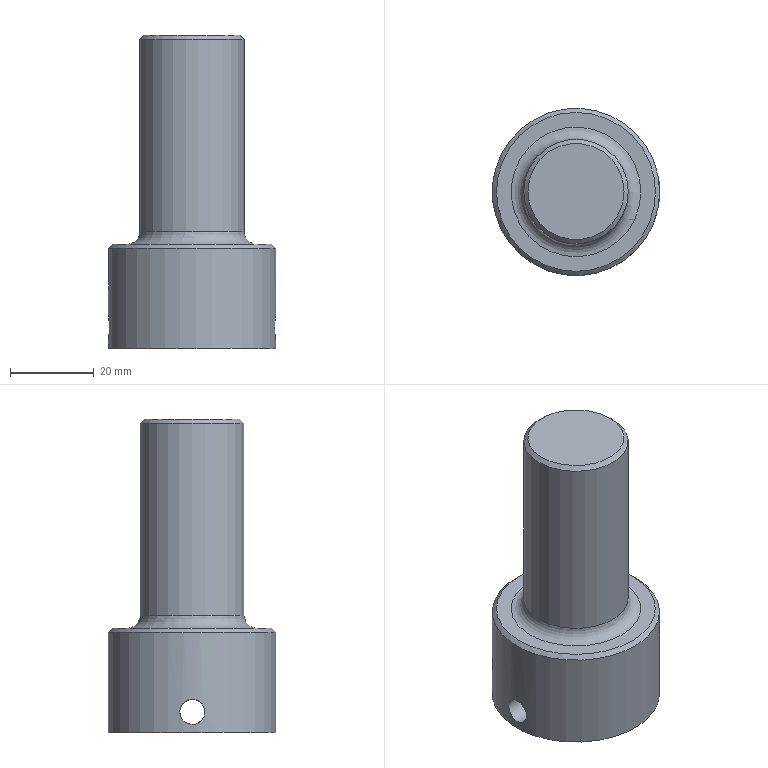Part | NX | features DATUM_CSYS 5, EXTRUDE 4, SKETCH 4, CHAMFER 2, BLEND 1 | 1 solid | 15 faces | box 40 x 40 x 75 mm | volume 54175 mm3 | plane 8 | cylinder 4 | cone 2 | torus 1 | commonest cylinder face diameters 6 x2 25 x1 40 x1
STEP:
#1=CARTESIAN_POINT('',(20.,0.,2.001));
#2=VERTEX_POINT('',#1);
#3=CARTESIAN_POINT('',(19.887,-2.373,2.578));
#4=CARTESIAN_POINT('',(20.056,0.01073,1.676));
#5=CARTESIAN_POINT('',(19.888,2.33,2.726));
#6=CARTESIAN_POINT('',(19.733,3.228,5.103));
#7=CARTESIAN_POINT('',(19.909,2.181,7.424));
#8=CARTESIAN_POINT('',(20.055,-0.2011,8.322));
#9=CARTESIAN_POINT('',(19.865,-2.516,7.277));
#10=CARTESIAN_POINT('',(19.701,-3.418,4.897));
#11=CARTESIAN_POINT('',(19.887,-2.373,2.578));
#12=CARTESIAN_POINT('',(20.056,0.01073,1.676));
#13=CARTESIAN_POINT('',(19.888,2.33,2.726));
#14=B_SPLINE_CURVE_WITH_KNOTS('',3,(#3,#4,#5,#6,#7,#8,#9,#10,#11,#12,#13),.UNSPECIFIED.,.T.,.F.,(1,1,1,1,1,1,1,1,1,1,1,1,1,1,1),(-0.007044,-0.004696,-0.002348,0.,0.002348,0.004696,0.007044,0.009392,0.01174,0.01409,0.01644,0.01878,0.02113,0.02348,0.02583),.UNSPECIFIED.);
#15=EDGE_CURVE('',#2,#2,#14,.T.);
#16=ORIENTED_EDGE('',*,*,#15,.F.);
#17=EDGE_LOOP('',(#16));
#18=FACE_BOUND('',#17,.T.);
#19=CARTESIAN_POINT('',(-20.,-0.0948,2.));
#20=VERTEX_POINT('',#19);
#21=CARTESIAN_POINT('',(-19.898,2.259,2.651));
#22=CARTESIAN_POINT('',(-20.056,-0.09565,1.675));
#23=CARTESIAN_POINT('',(-19.876,-2.445,2.65));
#24=CARTESIAN_POINT('',(-19.701,-3.419,4.996));
#25=CARTESIAN_POINT('',(-19.876,-2.447,7.35));
#26=CARTESIAN_POINT('',(-20.056,-0.09747,8.324));
#27=CARTESIAN_POINT('',(-19.899,2.253,7.354));
#28=CARTESIAN_POINT('',(-19.733,3.23,5.004));
#29=CARTESIAN_POINT('',(-19.898,2.259,2.651));
#30=CARTESIAN_POINT('',(-20.056,-0.09565,1.675));
#31=CARTESIAN_POINT('',(-19.876,-2.445,2.65));
#32=B_SPLINE_CURVE_WITH_KNOTS('',3,(#21,#22,#23,#24,#25,#26,#27,#28,#29,#30,#31),.UNSPECIFIED.,.T.,.F.,(1,1,1,1,1,1,1,1,1,1,1,1,1,1,1),(-0.007044,-0.004696,-0.002348,0.,0.002348,0.004696,0.007044,0.009391,0.01174,0.01409,0.01644,0.01878,0.02113,0.02348,0.02583),.UNSPECIFIED.);
#33=EDGE_CURVE('',#20,#20,#32,.T.);
#34=ORIENTED_EDGE('',*,*,#33,.F.);
#35=EDGE_LOOP('',(#34));
#36=FACE_BOUND('',#35,.T.);
#37=CARTESIAN_POINT('',(20.,0.,24.));
#38=VERTEX_POINT('',#37);
#39=CARTESIAN_POINT('',(0.,0.,24.));
#40=DIRECTION('',(0.,0.,1.));
#41=DIRECTION('',(1.,0.,0.));
#42=AXIS2_PLACEMENT_3D('',#39,#40,#41);
#43=CIRCLE('',#42,20.);
#44=EDGE_CURVE('',#38,#38,#43,.F.);
#45=ORIENTED_EDGE('',*,*,#44,.T.);
#46=EDGE_LOOP('',(#45));
#47=FACE_BOUND('',#46,.T.);
#48=CARTESIAN_POINT('',(20.,0.,0.));
#49=VERTEX_POINT('',#48);
#50=CARTESIAN_POINT('',(0.,0.,0.));
#51=DIRECTION('',(0.,0.,1.));
#52=DIRECTION('',(1.,0.,0.));
#53=AXIS2_PLACEMENT_3D('',#50,#51,#52);
#54=CIRCLE('',#53,20.);
#55=EDGE_CURVE('',#49,#49,#54,.T.);
#56=ORIENTED_EDGE('',*,*,#55,.T.);
#57=EDGE_LOOP('',(#56));
#58=FACE_BOUND('',#57,.T.);
#59=CARTESIAN_POINT('',(0.,0.,0.));
#60=DIRECTION('',(0.,0.,1.));
#61=DIRECTION('',(1.,0.,0.));
#62=AXIS2_PLACEMENT_3D('',#59,#60,#61);
#63=CYLINDRICAL_SURFACE('',#62,20.);
#64=ADVANCED_FACE('',(#18,#36,#47,#58),#63,.T.);
#65=CARTESIAN_POINT('',(5.,5.,0.));
#66=VERTEX_POINT('',#65);
#67=CARTESIAN_POINT('',(-5.,5.,0.));
#68=VERTEX_POINT('',#67);
#69=CARTESIAN_POINT('',(5.,5.,0.));
#70=DIRECTION('',(-1.,0.,0.));
#71=VECTOR('',#70,1000.);
#72=LINE('',#69,#71);
#73=EDGE_CURVE('',#66,#68,#72,.T.);
#74=ORIENTED_EDGE('',*,*,#73,.T.);
#75=CARTESIAN_POINT('',(-5.,-5.,0.));
#76=VERTEX_POINT('',#75);
#77=CARTESIAN_POINT('',(-5.,5.,0.));
#78=DIRECTION('',(0.,-1.,0.));
#79=VECTOR('',#78,1000.);
#80=LINE('',#77,#79);
#81=EDGE_CURVE('',#68,#76,#80,.T.);
#82=ORIENTED_EDGE('',*,*,#81,.T.);
#83=CARTESIAN_POINT('',(5.,-5.,0.));
#84=VERTEX_POINT('',#83);
#85=CARTESIAN_POINT('',(-5.,-5.,0.));
#86=DIRECTION('',(1.,0.,0.));
#87=VECTOR('',#86,1000.);
#88=LINE('',#85,#87);
#89=EDGE_CURVE('',#76,#84,#88,.T.);
#90=ORIENTED_EDGE('',*,*,#89,.T.);
#91=CARTESIAN_POINT('',(5.,-5.,0.));
#92=DIRECTION('',(0.,1.,0.));
#93=VECTOR('',#92,1000.);
#94=LINE('',#91,#93);
#95=EDGE_CURVE('',#84,#66,#94,.T.);
#96=ORIENTED_EDGE('',*,*,#95,.T.);
#97=EDGE_LOOP('',(#74,#82,#90,#96));
#98=FACE_BOUND('',#97,.T.);
#99=ORIENTED_EDGE('',*,*,#55,.F.);
#100=EDGE_LOOP('',(#99));
#101=FACE_BOUND('',#100,.T.);
#102=CARTESIAN_POINT('',(0.,0.,0.));
#103=DIRECTION('',(0.,0.,1.));
#104=DIRECTION('',(1.,0.,0.));
#105=AXIS2_PLACEMENT_3D('',#102,#103,#104);
#106=PLANE('',#105);
#107=ADVANCED_FACE('',(#98,#101),#106,.F.);
#108=CARTESIAN_POINT('',(15.5,0.,25.));
#109=VERTEX_POINT('',#108);
#110=CARTESIAN_POINT('',(0.,0.,25.));
#111=DIRECTION('',(0.,0.,1.));
#112=DIRECTION('',(1.,0.,0.));
#113=AXIS2_PLACEMENT_3D('',#110,#111,#112);
#114=CIRCLE('',#113,15.5);
#115=EDGE_CURVE('',#109,#109,#114,.F.);
#116=ORIENTED_EDGE('',*,*,#115,.T.);
#117=EDGE_LOOP('',(#116));
#118=FACE_BOUND('',#117,.T.);
#119=CARTESIAN_POINT('',(19.,0.,25.));
#120=VERTEX_POINT('',#119);
#121=CARTESIAN_POINT('',(0.,0.,25.));
#122=DIRECTION('',(0.,0.,1.));
#123=DIRECTION('',(1.,0.,0.));
#124=AXIS2_PLACEMENT_3D('',#121,#122,#123);
#125=CIRCLE('',#124,19.);
#126=EDGE_CURVE('',#120,#120,#125,.T.);
#127=ORIENTED_EDGE('',*,*,#126,.T.);
#128=EDGE_LOOP('',(#127));
#129=FACE_BOUND('',#128,.T.);
#130=CARTESIAN_POINT('',(0.,0.,25.));
#131=DIRECTION('',(0.,0.,1.));
#132=DIRECTION('',(1.,0.,0.));
#133=AXIS2_PLACEMENT_3D('',#130,#131,#132);
#134=PLANE('',#133);
#135=ADVANCED_FACE('',(#118,#129),#134,.T.);
#136=ORIENTED_EDGE('',*,*,#44,.F.);
#137=EDGE_LOOP('',(#136));
#138=FACE_BOUND('',#137,.T.);
#139=ORIENTED_EDGE('',*,*,#126,.F.);
#140=EDGE_LOOP('',(#139));
#141=FACE_BOUND('',#140,.T.);
#142=CARTESIAN_POINT('',(0.,0.,25.));
#143=DIRECTION('',(0.,0.,-1.));
#144=DIRECTION('',(-1.,0.,0.));
#145=AXIS2_PLACEMENT_3D('',#142,#143,#144);
#146=CONICAL_SURFACE('',#145,19.,0.7854);
#147=ADVANCED_FACE('',(#138,#141),#146,.T.);
#148=CARTESIAN_POINT('',(-5.,-3.095,5.));
#149=VERTEX_POINT('',#148);
#150=CARTESIAN_POINT('',(-5.,-0.0948,5.));
#151=DIRECTION('',(-1.,0.,0.));
#152=DIRECTION('',(0.,-1.,0.));
#153=AXIS2_PLACEMENT_3D('',#150,#151,#152);
#154=CIRCLE('',#153,3.);
#155=EDGE_CURVE('',#149,#149,#154,.T.);
#156=ORIENTED_EDGE('',*,*,#155,.T.);
#157=EDGE_LOOP('',(#156));
#158=FACE_BOUND('',#157,.T.);
#159=CARTESIAN_POINT('',(-5.,-5.,10.));
#160=VERTEX_POINT('',#159);
#161=CARTESIAN_POINT('',(-5.,5.,10.));
#162=VERTEX_POINT('',#161);
#163=CARTESIAN_POINT('',(-5.,5.,10.));
#164=DIRECTION('',(0.,-1.,0.));
#165=VECTOR('',#164,1000.);
#166=LINE('',#163,#165);
#167=EDGE_CURVE('',#160,#162,#166,.F.);
#168=ORIENTED_EDGE('',*,*,#167,.F.);
#169=CARTESIAN_POINT('',(-5.,-5.,0.));
#170=DIRECTION('',(0.,0.,1.));
#171=VECTOR('',#170,1000.);
#172=LINE('',#169,#171);
#173=EDGE_CURVE('',#160,#76,#172,.F.);
#174=ORIENTED_EDGE('',*,*,#173,.T.);
#175=ORIENTED_EDGE('',*,*,#81,.F.);
#176=CARTESIAN_POINT('',(-5.,5.,0.));
#177=DIRECTION('',(0.,0.,1.));
#178=VECTOR('',#177,1000.);
#179=LINE('',#176,#178);
#180=EDGE_CURVE('',#162,#68,#179,.F.);
#181=ORIENTED_EDGE('',*,*,#180,.F.);
#182=EDGE_LOOP('',(#168,#174,#175,#181));
#183=FACE_BOUND('',#182,.T.);
#184=CARTESIAN_POINT('',(-5.,5.,0.));
#185=DIRECTION('',(-1.,0.,0.));
#186=DIRECTION('',(0.,-1.,0.));
#187=AXIS2_PLACEMENT_3D('',#184,#185,#186);
#188=PLANE('',#187);
#189=ADVANCED_FACE('',(#158,#183),#188,.F.);
#190=CARTESIAN_POINT('',(5.,-5.,10.));
#191=VERTEX_POINT('',#190);
#192=CARTESIAN_POINT('',(-5.,-5.,10.));
#193=DIRECTION('',(1.,0.,0.));
#194=VECTOR('',#193,1000.);
#195=LINE('',#192,#194);
#196=EDGE_CURVE('',#191,#160,#195,.F.);
#197=ORIENTED_EDGE('',*,*,#196,.F.);
#198=CARTESIAN_POINT('',(5.,-5.,0.));
#199=DIRECTION('',(0.,0.,1.));
#200=VECTOR('',#199,1000.);
#201=LINE('',#198,#200);
#202=EDGE_CURVE('',#191,#84,#201,.F.);
#203=ORIENTED_EDGE('',*,*,#202,.T.);
#204=ORIENTED_EDGE('',*,*,#89,.F.);
#205=ORIENTED_EDGE('',*,*,#173,.F.);
#206=EDGE_LOOP('',(#197,#203,#204,#205));
#207=FACE_BOUND('',#206,.T.);
#208=CARTESIAN_POINT('',(-5.,-5.,0.));
#209=DIRECTION('',(0.,-1.,0.));
#210=DIRECTION('',(1.,0.,0.));
#211=AXIS2_PLACEMENT_3D('',#208,#209,#210);
#212=PLANE('',#211);
#213=ADVANCED_FACE('',(#207),#212,.F.);
#214=CARTESIAN_POINT('',(5.,2.905,5.));
#215=VERTEX_POINT('',#214);
#216=CARTESIAN_POINT('',(5.,-0.0948,5.));
#217=DIRECTION('',(1.,0.,0.));
#218=DIRECTION('',(0.,1.,0.));
#219=AXIS2_PLACEMENT_3D('',#216,#217,#218);
#220=CIRCLE('',#219,3.);
#221=EDGE_CURVE('',#215,#215,#220,.T.);
#222=ORIENTED_EDGE('',*,*,#221,.T.);
#223=EDGE_LOOP('',(#222));
#224=FACE_BOUND('',#223,.T.);
#225=CARTESIAN_POINT('',(5.,5.,10.));
#226=VERTEX_POINT('',#225);
#227=CARTESIAN_POINT('',(5.,-5.,10.));
#228=DIRECTION('',(0.,1.,0.));
#229=VECTOR('',#228,1000.);
#230=LINE('',#227,#229);
#231=EDGE_CURVE('',#226,#191,#230,.F.);
#232=ORIENTED_EDGE('',*,*,#231,.F.);
#233=CARTESIAN_POINT('',(5.,5.,0.));
#234=DIRECTION('',(0.,0.,1.));
#235=VECTOR('',#234,1000.);
#236=LINE('',#233,#235);
#237=EDGE_CURVE('',#226,#66,#236,.F.);
#238=ORIENTED_EDGE('',*,*,#237,.T.);
#239=ORIENTED_EDGE('',*,*,#95,.F.);
#240=ORIENTED_EDGE('',*,*,#202,.F.);
#241=EDGE_LOOP('',(#232,#238,#239,#240));
#242=FACE_BOUND('',#241,.T.);
#243=CARTESIAN_POINT('',(5.,-5.,0.));
#244=DIRECTION('',(1.,0.,0.));
#245=DIRECTION('',(0.,1.,0.));
#246=AXIS2_PLACEMENT_3D('',#243,#244,#245);
#247=PLANE('',#246);
#248=ADVANCED_FACE('',(#224,#242),#247,.F.);
#249=CARTESIAN_POINT('',(5.,5.,10.));
#250=DIRECTION('',(-1.,0.,0.));
#251=VECTOR('',#250,1000.);
#252=LINE('',#249,#251);
#253=EDGE_CURVE('',#162,#226,#252,.F.);
#254=ORIENTED_EDGE('',*,*,#253,.F.);
#255=ORIENTED_EDGE('',*,*,#180,.T.);
#256=ORIENTED_EDGE('',*,*,#73,.F.);
#257=ORIENTED_EDGE('',*,*,#237,.F.);
#258=EDGE_LOOP('',(#254,#255,#256,#257));
#259=FACE_BOUND('',#258,.T.);
#260=CARTESIAN_POINT('',(5.,5.,0.));
#261=DIRECTION('',(0.,1.,0.));
#262=DIRECTION('',(-1.,0.,0.));
#263=AXIS2_PLACEMENT_3D('',#260,#261,#262);
#264=PLANE('',#263);
#265=ADVANCED_FACE('',(#259),#264,.F.);
#266=ORIENTED_EDGE('',*,*,#167,.T.);
#267=ORIENTED_EDGE('',*,*,#253,.T.);
#268=ORIENTED_EDGE('',*,*,#231,.T.);
#269=ORIENTED_EDGE('',*,*,#196,.T.);
#270=EDGE_LOOP('',(#266,#267,#268,#269));
#271=FACE_BOUND('',#270,.T.);
#272=CARTESIAN_POINT('',(0.,0.,10.));
#273=DIRECTION('',(0.,0.,1.));
#274=DIRECTION('',(1.,0.,0.));
#275=AXIS2_PLACEMENT_3D('',#272,#273,#274);
#276=PLANE('',#275);
#277=ADVANCED_FACE('',(#271),#276,.F.);
#278=ORIENTED_EDGE('',*,*,#15,.T.);
#279=EDGE_LOOP('',(#278));
#280=FACE_BOUND('',#279,.T.);
#281=ORIENTED_EDGE('',*,*,#221,.F.);
#282=EDGE_LOOP('',(#281));
#283=FACE_BOUND('',#282,.T.);
#284=CARTESIAN_POINT('',(-24.5,-0.0948,5.));
#285=DIRECTION('',(1.,0.,0.));
#286=DIRECTION('',(0.,0.,-1.));
#287=AXIS2_PLACEMENT_3D('',#284,#285,#286);
#288=CYLINDRICAL_SURFACE('',#287,3.);
#289=ADVANCED_FACE('',(#280,#283),#288,.F.);
#290=ORIENTED_EDGE('',*,*,#33,.T.);
#291=EDGE_LOOP('',(#290));
#292=FACE_BOUND('',#291,.T.);
#293=ORIENTED_EDGE('',*,*,#155,.F.);
#294=EDGE_LOOP('',(#293));
#295=FACE_BOUND('',#294,.T.);
#296=CARTESIAN_POINT('',(-24.5,-0.0948,5.));
#297=DIRECTION('',(1.,0.,0.));
#298=DIRECTION('',(0.,0.,-1.));
#299=AXIS2_PLACEMENT_3D('',#296,#297,#298);
#300=CYLINDRICAL_SURFACE('',#299,3.);
#301=ADVANCED_FACE('',(#292,#295),#300,.F.);
#302=CARTESIAN_POINT('',(12.5,0.,74.));
#303=VERTEX_POINT('',#302);
#304=CARTESIAN_POINT('',(0.,0.,74.));
#305=DIRECTION('',(0.,0.,1.));
#306=DIRECTION('',(1.,0.,0.));
#307=AXIS2_PLACEMENT_3D('',#304,#305,#306);
#308=CIRCLE('',#307,12.5);
#309=EDGE_CURVE('',#303,#303,#308,.F.);
#310=ORIENTED_EDGE('',*,*,#309,.T.);
#311=EDGE_LOOP('',(#310));
#312=FACE_BOUND('',#311,.T.);
#313=CARTESIAN_POINT('',(12.5,0.,28.));
#314=VERTEX_POINT('',#313);
#315=CARTESIAN_POINT('',(0.,0.,28.));
#316=DIRECTION('',(0.,0.,1.));
#317=DIRECTION('',(1.,0.,0.));
#318=AXIS2_PLACEMENT_3D('',#315,#316,#317);
#319=CIRCLE('',#318,12.5);
#320=EDGE_CURVE('',#314,#314,#319,.T.);
#321=ORIENTED_EDGE('',*,*,#320,.T.);
#322=EDGE_LOOP('',(#321));
#323=FACE_BOUND('',#322,.T.);
#324=CARTESIAN_POINT('',(0.,0.,75.));
#325=DIRECTION('',(0.,0.,-1.));
#326=DIRECTION('',(-1.,0.,0.));
#327=AXIS2_PLACEMENT_3D('',#324,#325,#326);
#328=CYLINDRICAL_SURFACE('',#327,12.5);
#329=ADVANCED_FACE('',(#312,#323),#328,.T.);
#330=CARTESIAN_POINT('',(11.5,0.,75.));
#331=VERTEX_POINT('',#330);
#332=CARTESIAN_POINT('',(0.,0.,75.));
#333=DIRECTION('',(0.,0.,1.));
#334=DIRECTION('',(1.,0.,0.));
#335=AXIS2_PLACEMENT_3D('',#332,#333,#334);
#336=CIRCLE('',#335,11.5);
#337=EDGE_CURVE('',#331,#331,#336,.T.);
#338=ORIENTED_EDGE('',*,*,#337,.T.);
#339=EDGE_LOOP('',(#338));
#340=FACE_BOUND('',#339,.T.);
#341=CARTESIAN_POINT('',(0.,0.,75.));
#342=DIRECTION('',(0.,0.,1.));
#343=DIRECTION('',(1.,0.,0.));
#344=AXIS2_PLACEMENT_3D('',#341,#342,#343);
#345=PLANE('',#344);
#346=ADVANCED_FACE('',(#340),#345,.T.);
#347=ORIENTED_EDGE('',*,*,#115,.F.);
#348=EDGE_LOOP('',(#347));
#349=FACE_BOUND('',#348,.T.);
#350=ORIENTED_EDGE('',*,*,#320,.F.);
#351=EDGE_LOOP('',(#350));
#352=FACE_BOUND('',#351,.T.);
#353=CARTESIAN_POINT('',(0.,0.,28.));
#354=DIRECTION('',(0.,0.,1.));
#355=DIRECTION('',(1.,0.,0.));
#356=AXIS2_PLACEMENT_3D('',#353,#354,#355);
#357=TOROIDAL_SURFACE('',#356,15.5,3.);
#358=ADVANCED_FACE('',(#349,#352),#357,.F.);
#359=ORIENTED_EDGE('',*,*,#309,.F.);
#360=EDGE_LOOP('',(#359));
#361=FACE_BOUND('',#360,.T.);
#362=ORIENTED_EDGE('',*,*,#337,.F.);
#363=EDGE_LOOP('',(#362));
#364=FACE_BOUND('',#363,.T.);
#365=CARTESIAN_POINT('',(0.,0.,75.));
#366=DIRECTION('',(0.,0.,-1.));
#367=DIRECTION('',(-1.,0.,0.));
#368=AXIS2_PLACEMENT_3D('',#365,#366,#367);
#369=CONICAL_SURFACE('',#368,11.5,0.7854);
#370=ADVANCED_FACE('',(#361,#364),#369,.T.);
#371=CLOSED_SHELL('',(#64,#107,#135,#147,#189,#213,#248,#265,#277,#289,#301,#329,#346,#358,#370));
#372=MANIFOLD_SOLID_BREP('',#371);
#373=(LENGTH_UNIT()NAMED_UNIT(*)SI_UNIT(.MILLI.,.METRE.));
#374=UNCERTAINTY_MEASURE_WITH_UNIT(LENGTH_MEASURE(0.0508),#373,'','');
#375=(NAMED_UNIT(*)PLANE_ANGLE_UNIT()SI_UNIT($,.RADIAN.));
#376=(NAMED_UNIT(*)SI_UNIT($,.STERADIAN.)SOLID_ANGLE_UNIT());
#377=(GEOMETRIC_REPRESENTATION_CONTEXT(3)GLOBAL_UNCERTAINTY_ASSIGNED_CONTEXT((#374))GLOBAL_UNIT_ASSIGNED_CONTEXT((#373,#375,#376))REPRESENTATION_CONTEXT('',''));
#378=ADVANCED_BREP_SHAPE_REPRESENTATION('',(#372),#377);